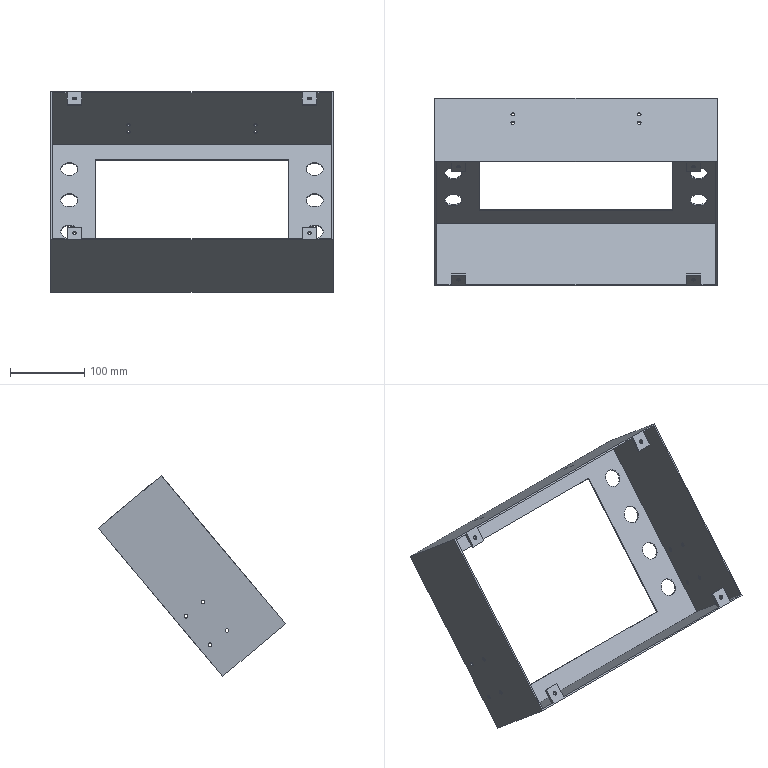Part | SolidWorks | features BaseBody 1 | 1 solid | 79 faces | box 380 x 251.39 x 269.878 mm | volume 364758 mm3 | cylinder 48 | plane 31 | commonest cylinder face diameters 5 x32 23 x16